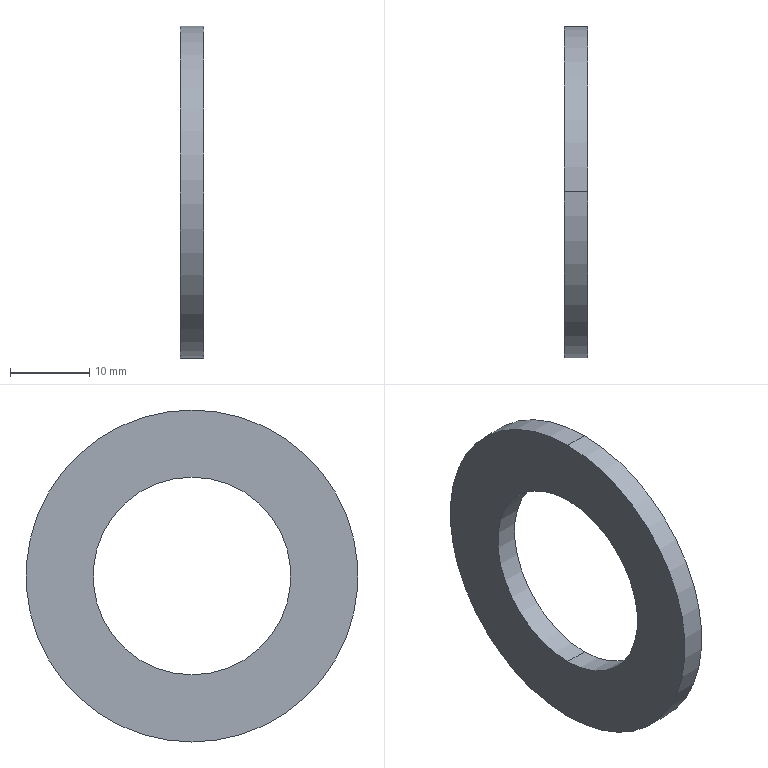Part | STEP file | Completa.sldasm-Part-114_Valor predeterminado | 1 solid | 6 faces | box 3 x 42 x 42 mm | volume 2684 mm3 | cylinder 4 | plane 2 | commonest cylinder face diameters 25 x2 42 x2
STEP:
#1=CARTESIAN_POINT('',(0.,0.,0.));
#2=DIRECTION('',(0.,0.,1.));
#3=DIRECTION('',(1.,0.,0.));
#4=AXIS2_PLACEMENT_3D('',#1,#2,#3);
#5=CARTESIAN_POINT('',(-53.103,0.,-21.));
#6=VERTEX_POINT('',#5);
#7=CARTESIAN_POINT('',(-53.103,0.,21.));
#8=VERTEX_POINT('',#7);
#9=CARTESIAN_POINT('',(-53.103,0.,0.));
#10=DIRECTION('',(1.,0.,0.));
#11=DIRECTION('',(0.,0.,1.));
#12=AXIS2_PLACEMENT_3D('',#9,#10,#11);
#13=CIRCLE('',#12,21.);
#14=CARTESIAN_POINT('',(-53.103,0.,0.));
#15=DIRECTION('',(-1.,0.,0.));
#16=DIRECTION('',(0.,0.,1.));
#17=AXIS2_PLACEMENT_3D('',#14,#15,#16);
#18=CYLINDRICAL_SURFACE('',#17,21.);
#19=CARTESIAN_POINT('',(6.283,0.));
#20=DIRECTION('',(-1.,0.));
#21=VECTOR('',#20,1.);
#22=LINE('',#19,#21);
#23=(GEOMETRIC_REPRESENTATION_CONTEXT(2)PARAMETRIC_REPRESENTATION_CONTEXT()REPRESENTATION_CONTEXT('',''));
#24=DEFINITIONAL_REPRESENTATION('',(#22),#23);
#25=PCURVE('',#18,#24);
#26=CARTESIAN_POINT('',(-53.103,0.,0.));
#27=DIRECTION('',(-1.,0.,0.));
#28=DIRECTION('',(0.,0.,1.));
#29=AXIS2_PLACEMENT_3D('',#26,#27,#28);
#30=PLANE('',#29);
#31=CARTESIAN_POINT('',(21.,0.));
#32=CARTESIAN_POINT('',(21.,-36.373));
#33=CARTESIAN_POINT('',(-10.5,-18.187));
#34=CARTESIAN_POINT('',(-42.,0.));
#35=CARTESIAN_POINT('',(-10.5,18.187));
#36=CARTESIAN_POINT('',(21.,36.373));
#37=CARTESIAN_POINT('',(21.,0.));
#38=(BOUNDED_CURVE()B_SPLINE_CURVE(2,(#31,#32,#33,#34,#35,#36,#37),.UNSPECIFIED.,.T.,.F.)B_SPLINE_CURVE_WITH_KNOTS((1,2,2,2,2,1),(-2.094,0.,2.094,4.189,6.283,8.378),.UNSPECIFIED.)CURVE()GEOMETRIC_REPRESENTATION_ITEM()RATIONAL_B_SPLINE_CURVE((1.,0.5,1.,0.5,1.,0.5,1.))REPRESENTATION_ITEM(''));
#39=(GEOMETRIC_REPRESENTATION_CONTEXT(2)PARAMETRIC_REPRESENTATION_CONTEXT()REPRESENTATION_CONTEXT('',''));
#40=DEFINITIONAL_REPRESENTATION('',(#38),#39);
#41=PCURVE('',#30,#40);
#42=SURFACE_CURVE('',#13,(#25,#41),.PCURVE_S1.);
#43=EDGE_CURVE('',#6,#8,#42,.T.);
#44=ORIENTED_EDGE('',*,*,#43,.F.);
#45=CARTESIAN_POINT('',(-56.103,0.,-21.));
#46=VERTEX_POINT('',#45);
#47=CARTESIAN_POINT('',(-53.103,0.,-21.));
#48=DIRECTION('',(-1.,0.,0.));
#49=VECTOR('',#48,1.);
#50=LINE('',#47,#49);
#51=CARTESIAN_POINT('',(3.142,0.));
#52=DIRECTION('',(0.,1.));
#53=VECTOR('',#52,1.);
#54=LINE('',#51,#53);
#55=(GEOMETRIC_REPRESENTATION_CONTEXT(2)PARAMETRIC_REPRESENTATION_CONTEXT()REPRESENTATION_CONTEXT('',''));
#56=DEFINITIONAL_REPRESENTATION('',(#54),#55);
#57=PCURVE('',#18,#56);
#58=CARTESIAN_POINT('',(-53.103,0.,0.));
#59=DIRECTION('',(-1.,0.,0.));
#60=DIRECTION('',(0.,0.,1.));
#61=AXIS2_PLACEMENT_3D('',#58,#59,#60);
#62=CYLINDRICAL_SURFACE('',#61,21.);
#63=CARTESIAN_POINT('',(3.142,0.));
#64=DIRECTION('',(0.,1.));
#65=VECTOR('',#64,1.);
#66=LINE('',#63,#65);
#67=(GEOMETRIC_REPRESENTATION_CONTEXT(2)PARAMETRIC_REPRESENTATION_CONTEXT()REPRESENTATION_CONTEXT('',''));
#68=DEFINITIONAL_REPRESENTATION('',(#66),#67);
#69=PCURVE('',#62,#68);
#70=SURFACE_CURVE('',#50,(#57,#69),.PCURVE_S1.);
#71=EDGE_CURVE('',#6,#46,#70,.T.);
#72=ORIENTED_EDGE('',*,*,#71,.T.);
#73=CARTESIAN_POINT('',(-56.103,0.,21.));
#74=VERTEX_POINT('',#73);
#75=CARTESIAN_POINT('',(-56.103,0.,0.));
#76=DIRECTION('',(1.,0.,0.));
#77=DIRECTION('',(0.,0.,1.));
#78=AXIS2_PLACEMENT_3D('',#75,#76,#77);
#79=CIRCLE('',#78,21.);
#80=CARTESIAN_POINT('',(6.283,3.));
#81=DIRECTION('',(-1.,0.));
#82=VECTOR('',#81,1.);
#83=LINE('',#80,#82);
#84=(GEOMETRIC_REPRESENTATION_CONTEXT(2)PARAMETRIC_REPRESENTATION_CONTEXT()REPRESENTATION_CONTEXT('',''));
#85=DEFINITIONAL_REPRESENTATION('',(#83),#84);
#86=PCURVE('',#18,#85);
#87=CARTESIAN_POINT('',(-56.103,0.,0.));
#88=DIRECTION('',(-1.,0.,0.));
#89=DIRECTION('',(0.,0.,1.));
#90=AXIS2_PLACEMENT_3D('',#87,#88,#89);
#91=PLANE('',#90);
#92=CARTESIAN_POINT('',(21.,0.));
#93=CARTESIAN_POINT('',(21.,-36.373));
#94=CARTESIAN_POINT('',(-10.5,-18.187));
#95=CARTESIAN_POINT('',(-42.,0.));
#96=CARTESIAN_POINT('',(-10.5,18.187));
#97=CARTESIAN_POINT('',(21.,36.373));
#98=CARTESIAN_POINT('',(21.,0.));
#99=(BOUNDED_CURVE()B_SPLINE_CURVE(2,(#92,#93,#94,#95,#96,#97,#98),.UNSPECIFIED.,.T.,.F.)B_SPLINE_CURVE_WITH_KNOTS((1,2,2,2,2,1),(-2.094,0.,2.094,4.189,6.283,8.378),.UNSPECIFIED.)CURVE()GEOMETRIC_REPRESENTATION_ITEM()RATIONAL_B_SPLINE_CURVE((1.,0.5,1.,0.5,1.,0.5,1.))REPRESENTATION_ITEM(''));
#100=(GEOMETRIC_REPRESENTATION_CONTEXT(2)PARAMETRIC_REPRESENTATION_CONTEXT()REPRESENTATION_CONTEXT('',''));
#101=DEFINITIONAL_REPRESENTATION('',(#99),#100);
#102=PCURVE('',#91,#101);
#103=SURFACE_CURVE('',#79,(#86,#102),.PCURVE_S1.);
#104=EDGE_CURVE('',#46,#74,#103,.T.);
#105=ORIENTED_EDGE('',*,*,#104,.T.);
#106=CARTESIAN_POINT('',(-53.103,0.,21.));
#107=DIRECTION('',(-1.,0.,0.));
#108=VECTOR('',#107,1.);
#109=LINE('',#106,#108);
#110=CARTESIAN_POINT('',(0.,0.));
#111=DIRECTION('',(0.,1.));
#112=VECTOR('',#111,1.);
#113=LINE('',#110,#112);
#114=(GEOMETRIC_REPRESENTATION_CONTEXT(2)PARAMETRIC_REPRESENTATION_CONTEXT()REPRESENTATION_CONTEXT('',''));
#115=DEFINITIONAL_REPRESENTATION('',(#113),#114);
#116=PCURVE('',#18,#115);
#117=CARTESIAN_POINT('',(6.283,0.));
#118=DIRECTION('',(0.,1.));
#119=VECTOR('',#118,1.);
#120=LINE('',#117,#119);
#121=(GEOMETRIC_REPRESENTATION_CONTEXT(2)PARAMETRIC_REPRESENTATION_CONTEXT()REPRESENTATION_CONTEXT('',''));
#122=DEFINITIONAL_REPRESENTATION('',(#120),#121);
#123=PCURVE('',#62,#122);
#124=SURFACE_CURVE('',#109,(#116,#123),.PCURVE_S1.);
#125=EDGE_CURVE('',#8,#74,#124,.T.);
#126=ORIENTED_EDGE('',*,*,#125,.F.);
#127=EDGE_LOOP('',(#44,#72,#105,#126));
#128=FACE_BOUND('',#127,.T.);
#129=ADVANCED_FACE('',(#128),#18,.T.);
#130=CARTESIAN_POINT('',(-53.103,0.,12.5));
#131=VERTEX_POINT('',#130);
#132=CARTESIAN_POINT('',(-56.103,0.,12.5));
#133=VERTEX_POINT('',#132);
#134=CARTESIAN_POINT('',(-53.103,0.,12.5));
#135=DIRECTION('',(-1.,0.,0.));
#136=VECTOR('',#135,1.);
#137=LINE('',#134,#136);
#138=CARTESIAN_POINT('',(-53.103,0.,0.));
#139=DIRECTION('',(-1.,0.,0.));
#140=DIRECTION('',(0.,0.,1.));
#141=AXIS2_PLACEMENT_3D('',#138,#139,#140);
#142=CYLINDRICAL_SURFACE('',#141,12.5);
#143=CARTESIAN_POINT('',(6.283,0.));
#144=DIRECTION('',(0.,1.));
#145=VECTOR('',#144,1.);
#146=LINE('',#143,#145);
#147=(GEOMETRIC_REPRESENTATION_CONTEXT(2)PARAMETRIC_REPRESENTATION_CONTEXT()REPRESENTATION_CONTEXT('',''));
#148=DEFINITIONAL_REPRESENTATION('',(#146),#147);
#149=PCURVE('',#142,#148);
#150=CARTESIAN_POINT('',(-53.103,0.,0.));
#151=DIRECTION('',(-1.,0.,0.));
#152=DIRECTION('',(0.,0.,1.));
#153=AXIS2_PLACEMENT_3D('',#150,#151,#152);
#154=CYLINDRICAL_SURFACE('',#153,12.5);
#155=CARTESIAN_POINT('',(0.,0.));
#156=DIRECTION('',(0.,1.));
#157=VECTOR('',#156,1.);
#158=LINE('',#155,#157);
#159=(GEOMETRIC_REPRESENTATION_CONTEXT(2)PARAMETRIC_REPRESENTATION_CONTEXT()REPRESENTATION_CONTEXT('',''));
#160=DEFINITIONAL_REPRESENTATION('',(#158),#159);
#161=PCURVE('',#154,#160);
#162=SURFACE_CURVE('',#137,(#149,#161),.PCURVE_S1.);
#163=EDGE_CURVE('',#131,#133,#162,.T.);
#164=ORIENTED_EDGE('',*,*,#163,.T.);
#165=CARTESIAN_POINT('',(-56.103,0.,-12.5));
#166=VERTEX_POINT('',#165);
#167=CARTESIAN_POINT('',(-56.103,0.,0.));
#168=DIRECTION('',(1.,0.,0.));
#169=DIRECTION('',(0.,0.,1.));
#170=AXIS2_PLACEMENT_3D('',#167,#168,#169);
#171=CIRCLE('',#170,12.5);
#172=CARTESIAN_POINT('',(6.283,3.));
#173=DIRECTION('',(-1.,0.));
#174=VECTOR('',#173,1.);
#175=LINE('',#172,#174);
#176=(GEOMETRIC_REPRESENTATION_CONTEXT(2)PARAMETRIC_REPRESENTATION_CONTEXT()REPRESENTATION_CONTEXT('',''));
#177=DEFINITIONAL_REPRESENTATION('',(#175),#176);
#178=PCURVE('',#142,#177);
#179=CARTESIAN_POINT('',(12.5,0.));
#180=CARTESIAN_POINT('',(12.5,-21.651));
#181=CARTESIAN_POINT('',(-6.25,-10.825));
#182=CARTESIAN_POINT('',(-25.,0.));
#183=CARTESIAN_POINT('',(-6.25,10.825));
#184=CARTESIAN_POINT('',(12.5,21.651));
#185=CARTESIAN_POINT('',(12.5,0.));
#186=(BOUNDED_CURVE()B_SPLINE_CURVE(2,(#179,#180,#181,#182,#183,#184,#185),.UNSPECIFIED.,.T.,.F.)B_SPLINE_CURVE_WITH_KNOTS((1,2,2,2,2,1),(-2.094,0.,2.094,4.189,6.283,8.378),.UNSPECIFIED.)CURVE()GEOMETRIC_REPRESENTATION_ITEM()RATIONAL_B_SPLINE_CURVE((1.,0.5,1.,0.5,1.,0.5,1.))REPRESENTATION_ITEM(''));
#187=(GEOMETRIC_REPRESENTATION_CONTEXT(2)PARAMETRIC_REPRESENTATION_CONTEXT()REPRESENTATION_CONTEXT('',''));
#188=DEFINITIONAL_REPRESENTATION('',(#186),#187);
#189=PCURVE('',#91,#188);
#190=SURFACE_CURVE('',#171,(#178,#189),.PCURVE_S1.);
#191=EDGE_CURVE('',#133,#166,#190,.T.);
#192=ORIENTED_EDGE('',*,*,#191,.T.);
#193=CARTESIAN_POINT('',(-53.103,0.,-12.5));
#194=VERTEX_POINT('',#193);
#195=CARTESIAN_POINT('',(-53.103,0.,-12.5));
#196=DIRECTION('',(-1.,0.,0.));
#197=VECTOR('',#196,1.);
#198=LINE('',#195,#197);
#199=CARTESIAN_POINT('',(3.142,0.));
#200=DIRECTION('',(0.,1.));
#201=VECTOR('',#200,1.);
#202=LINE('',#199,#201);
#203=(GEOMETRIC_REPRESENTATION_CONTEXT(2)PARAMETRIC_REPRESENTATION_CONTEXT()REPRESENTATION_CONTEXT('',''));
#204=DEFINITIONAL_REPRESENTATION('',(#202),#203);
#205=PCURVE('',#142,#204);
#206=CARTESIAN_POINT('',(3.142,0.));
#207=DIRECTION('',(0.,1.));
#208=VECTOR('',#207,1.);
#209=LINE('',#206,#208);
#210=(GEOMETRIC_REPRESENTATION_CONTEXT(2)PARAMETRIC_REPRESENTATION_CONTEXT()REPRESENTATION_CONTEXT('',''));
#211=DEFINITIONAL_REPRESENTATION('',(#209),#210);
#212=PCURVE('',#154,#211);
#213=SURFACE_CURVE('',#198,(#205,#212),.PCURVE_S1.);
#214=EDGE_CURVE('',#194,#166,#213,.T.);
#215=ORIENTED_EDGE('',*,*,#214,.F.);
#216=CARTESIAN_POINT('',(-53.103,0.,0.));
#217=DIRECTION('',(1.,0.,0.));
#218=DIRECTION('',(0.,0.,1.));
#219=AXIS2_PLACEMENT_3D('',#216,#217,#218);
#220=CIRCLE('',#219,12.5);
#221=CARTESIAN_POINT('',(6.283,0.));
#222=DIRECTION('',(-1.,0.));
#223=VECTOR('',#222,1.);
#224=LINE('',#221,#223);
#225=(GEOMETRIC_REPRESENTATION_CONTEXT(2)PARAMETRIC_REPRESENTATION_CONTEXT()REPRESENTATION_CONTEXT('',''));
#226=DEFINITIONAL_REPRESENTATION('',(#224),#225);
#227=PCURVE('',#142,#226);
#228=CARTESIAN_POINT('',(12.5,0.));
#229=CARTESIAN_POINT('',(12.5,-21.651));
#230=CARTESIAN_POINT('',(-6.25,-10.825));
#231=CARTESIAN_POINT('',(-25.,0.));
#232=CARTESIAN_POINT('',(-6.25,10.825));
#233=CARTESIAN_POINT('',(12.5,21.651));
#234=CARTESIAN_POINT('',(12.5,0.));
#235=(BOUNDED_CURVE()B_SPLINE_CURVE(2,(#228,#229,#230,#231,#232,#233,#234),.UNSPECIFIED.,.T.,.F.)B_SPLINE_CURVE_WITH_KNOTS((1,2,2,2,2,1),(-2.094,0.,2.094,4.189,6.283,8.378),.UNSPECIFIED.)CURVE()GEOMETRIC_REPRESENTATION_ITEM()RATIONAL_B_SPLINE_CURVE((1.,0.5,1.,0.5,1.,0.5,1.))REPRESENTATION_ITEM(''));
#236=(GEOMETRIC_REPRESENTATION_CONTEXT(2)PARAMETRIC_REPRESENTATION_CONTEXT()REPRESENTATION_CONTEXT('',''));
#237=DEFINITIONAL_REPRESENTATION('',(#235),#236);
#238=PCURVE('',#30,#237);
#239=SURFACE_CURVE('',#220,(#227,#238),.PCURVE_S1.);
#240=EDGE_CURVE('',#131,#194,#239,.T.);
#241=ORIENTED_EDGE('',*,*,#240,.F.);
#242=EDGE_LOOP('',(#164,#192,#215,#241));
#243=FACE_BOUND('',#242,.F.);
#244=ADVANCED_FACE('',(#243),#142,.F.);
#245=ORIENTED_EDGE('',*,*,#240,.F.);
#246=CARTESIAN_POINT('',(-53.103,0.,0.));
#247=DIRECTION('',(1.,0.,0.));
#248=DIRECTION('',(0.,0.,1.));
#249=AXIS2_PLACEMENT_3D('',#246,#247,#248);
#250=CIRCLE('',#249,12.5);
#251=CARTESIAN_POINT('',(12.5,0.));
#252=CARTESIAN_POINT('',(12.5,-21.651));
#253=CARTESIAN_POINT('',(-6.25,-10.825));
#254=CARTESIAN_POINT('',(-25.,0.));
#255=CARTESIAN_POINT('',(-6.25,10.825));
#256=CARTESIAN_POINT('',(12.5,21.651));
#257=CARTESIAN_POINT('',(12.5,0.));
#258=(BOUNDED_CURVE()B_SPLINE_CURVE(2,(#251,#252,#253,#254,#255,#256,#257),.UNSPECIFIED.,.T.,.F.)B_SPLINE_CURVE_WITH_KNOTS((1,2,2,2,2,1),(-2.094,0.,2.094,4.189,6.283,8.378),.UNSPECIFIED.)CURVE()GEOMETRIC_REPRESENTATION_ITEM()RATIONAL_B_SPLINE_CURVE((1.,0.5,1.,0.5,1.,0.5,1.))REPRESENTATION_ITEM(''));
#259=(GEOMETRIC_REPRESENTATION_CONTEXT(2)PARAMETRIC_REPRESENTATION_CONTEXT()REPRESENTATION_CONTEXT('',''));
#260=DEFINITIONAL_REPRESENTATION('',(#258),#259);
#261=PCURVE('',#30,#260);
#262=CARTESIAN_POINT('',(6.283,0.));
#263=DIRECTION('',(-1.,0.));
#264=VECTOR('',#263,1.);
#265=LINE('',#262,#264);
#266=(GEOMETRIC_REPRESENTATION_CONTEXT(2)PARAMETRIC_REPRESENTATION_CONTEXT()REPRESENTATION_CONTEXT('',''));
#267=DEFINITIONAL_REPRESENTATION('',(#265),#266);
#268=PCURVE('',#154,#267);
#269=SURFACE_CURVE('',#250,(#261,#268),.PCURVE_S1.);
#270=EDGE_CURVE('',#194,#131,#269,.T.);
#271=ORIENTED_EDGE('',*,*,#270,.F.);
#272=EDGE_LOOP('',(#245,#271));
#273=FACE_BOUND('',#272,.T.);
#274=CARTESIAN_POINT('',(-53.103,0.,0.));
#275=DIRECTION('',(1.,0.,0.));
#276=DIRECTION('',(0.,0.,1.));
#277=AXIS2_PLACEMENT_3D('',#274,#275,#276);
#278=CIRCLE('',#277,21.);
#279=CARTESIAN_POINT('',(21.,0.));
#280=CARTESIAN_POINT('',(21.,-36.373));
#281=CARTESIAN_POINT('',(-10.5,-18.187));
#282=CARTESIAN_POINT('',(-42.,0.));
#283=CARTESIAN_POINT('',(-10.5,18.187));
#284=CARTESIAN_POINT('',(21.,36.373));
#285=CARTESIAN_POINT('',(21.,0.));
#286=(BOUNDED_CURVE()B_SPLINE_CURVE(2,(#279,#280,#281,#282,#283,#284,#285),.UNSPECIFIED.,.T.,.F.)B_SPLINE_CURVE_WITH_KNOTS((1,2,2,2,2,1),(-2.094,0.,2.094,4.189,6.283,8.378),.UNSPECIFIED.)CURVE()GEOMETRIC_REPRESENTATION_ITEM()RATIONAL_B_SPLINE_CURVE((1.,0.5,1.,0.5,1.,0.5,1.))REPRESENTATION_ITEM(''));
#287=(GEOMETRIC_REPRESENTATION_CONTEXT(2)PARAMETRIC_REPRESENTATION_CONTEXT()REPRESENTATION_CONTEXT('',''));
#288=DEFINITIONAL_REPRESENTATION('',(#286),#287);
#289=PCURVE('',#30,#288);
#290=CARTESIAN_POINT('',(6.283,0.));
#291=DIRECTION('',(-1.,0.));
#292=VECTOR('',#291,1.);
#293=LINE('',#290,#292);
#294=(GEOMETRIC_REPRESENTATION_CONTEXT(2)PARAMETRIC_REPRESENTATION_CONTEXT()REPRESENTATION_CONTEXT('',''));
#295=DEFINITIONAL_REPRESENTATION('',(#293),#294);
#296=PCURVE('',#62,#295);
#297=SURFACE_CURVE('',#278,(#289,#296),.PCURVE_S1.);
#298=EDGE_CURVE('',#8,#6,#297,.T.);
#299=ORIENTED_EDGE('',*,*,#298,.T.);
#300=ORIENTED_EDGE('',*,*,#43,.T.);
#301=EDGE_LOOP('',(#299,#300));
#302=FACE_BOUND('',#301,.T.);
#303=ADVANCED_FACE('',(#273,#302),#30,.F.);
#304=ORIENTED_EDGE('',*,*,#191,.T.);
#305=CARTESIAN_POINT('',(-56.103,0.,0.));
#306=DIRECTION('',(1.,0.,0.));
#307=DIRECTION('',(0.,0.,1.));
#308=AXIS2_PLACEMENT_3D('',#305,#306,#307);
#309=CIRCLE('',#308,12.5);
#310=CARTESIAN_POINT('',(12.5,0.));
#311=CARTESIAN_POINT('',(12.5,-21.651));
#312=CARTESIAN_POINT('',(-6.25,-10.825));
#313=CARTESIAN_POINT('',(-25.,0.));
#314=CARTESIAN_POINT('',(-6.25,10.825));
#315=CARTESIAN_POINT('',(12.5,21.651));
#316=CARTESIAN_POINT('',(12.5,0.));
#317=(BOUNDED_CURVE()B_SPLINE_CURVE(2,(#310,#311,#312,#313,#314,#315,#316),.UNSPECIFIED.,.T.,.F.)B_SPLINE_CURVE_WITH_KNOTS((1,2,2,2,2,1),(-2.094,0.,2.094,4.189,6.283,8.378),.UNSPECIFIED.)CURVE()GEOMETRIC_REPRESENTATION_ITEM()RATIONAL_B_SPLINE_CURVE((1.,0.5,1.,0.5,1.,0.5,1.))REPRESENTATION_ITEM(''));
#318=(GEOMETRIC_REPRESENTATION_CONTEXT(2)PARAMETRIC_REPRESENTATION_CONTEXT()REPRESENTATION_CONTEXT('',''));
#319=DEFINITIONAL_REPRESENTATION('',(#317),#318);
#320=PCURVE('',#91,#319);
#321=CARTESIAN_POINT('',(6.283,3.));
#322=DIRECTION('',(-1.,0.));
#323=VECTOR('',#322,1.);
#324=LINE('',#321,#323);
#325=(GEOMETRIC_REPRESENTATION_CONTEXT(2)PARAMETRIC_REPRESENTATION_CONTEXT()REPRESENTATION_CONTEXT('',''));
#326=DEFINITIONAL_REPRESENTATION('',(#324),#325);
#327=PCURVE('',#154,#326);
#328=SURFACE_CURVE('',#309,(#320,#327),.PCURVE_S1.);
#329=EDGE_CURVE('',#166,#133,#328,.T.);
#330=ORIENTED_EDGE('',*,*,#329,.T.);
#331=EDGE_LOOP('',(#304,#330));
#332=FACE_BOUND('',#331,.T.);
#333=CARTESIAN_POINT('',(-56.103,0.,0.));
#334=DIRECTION('',(1.,0.,0.));
#335=DIRECTION('',(0.,0.,1.));
#336=AXIS2_PLACEMENT_3D('',#333,#334,#335);
#337=CIRCLE('',#336,21.);
#338=CARTESIAN_POINT('',(21.,0.));
#339=CARTESIAN_POINT('',(21.,-36.373));
#340=CARTESIAN_POINT('',(-10.5,-18.187));
#341=CARTESIAN_POINT('',(-42.,0.));
#342=CARTESIAN_POINT('',(-10.5,18.187));
#343=CARTESIAN_POINT('',(21.,36.373));
#344=CARTESIAN_POINT('',(21.,0.));
#345=(BOUNDED_CURVE()B_SPLINE_CURVE(2,(#338,#339,#340,#341,#342,#343,#344),.UNSPECIFIED.,.T.,.F.)B_SPLINE_CURVE_WITH_KNOTS((1,2,2,2,2,1),(-2.094,0.,2.094,4.189,6.283,8.378),.UNSPECIFIED.)CURVE()GEOMETRIC_REPRESENTATION_ITEM()RATIONAL_B_SPLINE_CURVE((1.,0.5,1.,0.5,1.,0.5,1.))REPRESENTATION_ITEM(''));
#346=(GEOMETRIC_REPRESENTATION_CONTEXT(2)PARAMETRIC_REPRESENTATION_CONTEXT()REPRESENTATION_CONTEXT('',''));
#347=DEFINITIONAL_REPRESENTATION('',(#345),#346);
#348=PCURVE('',#91,#347);
#349=CARTESIAN_POINT('',(6.283,3.));
#350=DIRECTION('',(-1.,0.));
#351=VECTOR('',#350,1.);
#352=LINE('',#349,#351);
#353=(GEOMETRIC_REPRESENTATION_CONTEXT(2)PARAMETRIC_REPRESENTATION_CONTEXT()REPRESENTATION_CONTEXT('',''));
#354=DEFINITIONAL_REPRESENTATION('',(#352),#353);
#355=PCURVE('',#62,#354);
#356=SURFACE_CURVE('',#337,(#348,#355),.PCURVE_S1.);
#357=EDGE_CURVE('',#74,#46,#356,.T.);
#358=ORIENTED_EDGE('',*,*,#357,.F.);
#359=ORIENTED_EDGE('',*,*,#104,.F.);
#360=EDGE_LOOP('',(#358,#359));
#361=FACE_BOUND('',#360,.T.);
#362=ADVANCED_FACE('',(#332,#361),#91,.T.);
#363=ORIENTED_EDGE('',*,*,#329,.T.);
#364=ORIENTED_EDGE('',*,*,#163,.F.);
#365=ORIENTED_EDGE('',*,*,#270,.F.);
#366=ORIENTED_EDGE('',*,*,#214,.T.);
#367=EDGE_LOOP('',(#363,#364,#365,#366));
#368=FACE_BOUND('',#367,.F.);
#369=ADVANCED_FACE('',(#368),#154,.F.);
#370=ORIENTED_EDGE('',*,*,#71,.F.);
#371=ORIENTED_EDGE('',*,*,#298,.F.);
#372=ORIENTED_EDGE('',*,*,#125,.T.);
#373=ORIENTED_EDGE('',*,*,#357,.T.);
#374=EDGE_LOOP('',(#370,#371,#372,#373));
#375=FACE_BOUND('',#374,.T.);
#376=ADVANCED_FACE('',(#375),#62,.T.);
#377=CLOSED_SHELL('',(#129,#244,#303,#362,#369,#376));
#378=MANIFOLD_SOLID_BREP('',#377);
#379=(LENGTH_UNIT()NAMED_UNIT(*)SI_UNIT(.MILLI.,.METRE.));
#380=UNCERTAINTY_MEASURE_WITH_UNIT(LENGTH_MEASURE(0.0000001),#379,'','');
#381=(NAMED_UNIT(*)PLANE_ANGLE_UNIT()SI_UNIT($,.RADIAN.));
#382=(NAMED_UNIT(*)SI_UNIT($,.STERADIAN.)SOLID_ANGLE_UNIT());
#383=(GEOMETRIC_REPRESENTATION_CONTEXT(3)GLOBAL_UNCERTAINTY_ASSIGNED_CONTEXT((#380))GLOBAL_UNIT_ASSIGNED_CONTEXT((#379,#381,#382))REPRESENTATION_CONTEXT('',''));
#384=ADVANCED_BREP_SHAPE_REPRESENTATION('',(#4,#378),#383);